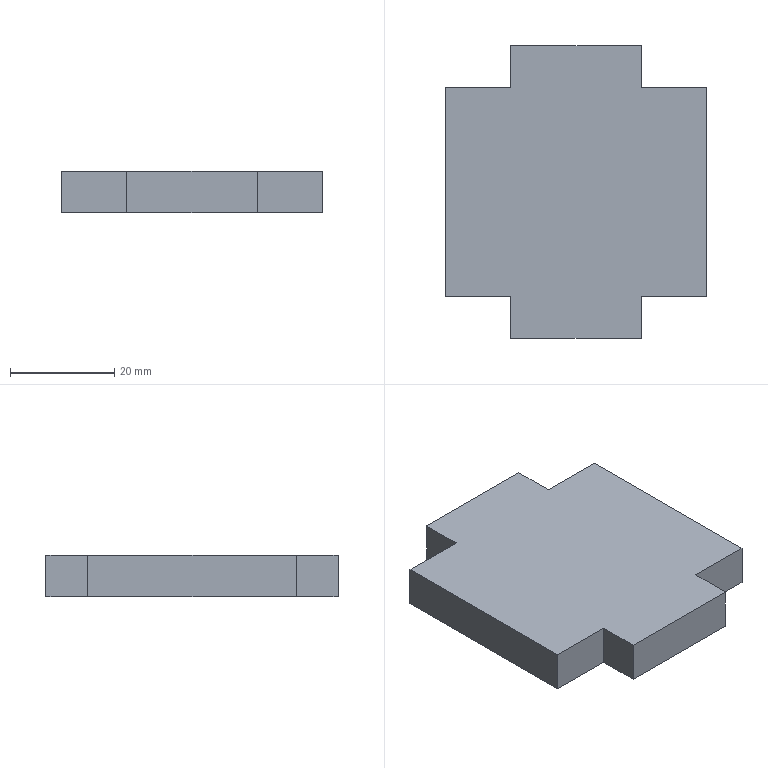Part | SolidWorks | features FlatPattern 1, SMBaseFlange 1, SheetMetal 1 | 1 solid | 14 faces | box 50 x 56 x 8 mm | volume 19200 mm3 | plane 14
STEP:
#1=CARTESIAN_POINT('',(361.372,8.,0.));
#2=VERTEX_POINT('',#1);
#3=CARTESIAN_POINT('',(373.872,8.,0.));
#4=VERTEX_POINT('',#3);
#5=CARTESIAN_POINT('',(373.872,8.,0.));
#6=DIRECTION('',(1.,0.,0.));
#7=VECTOR('',#6,1000.);
#8=LINE('',#5,#7);
#9=EDGE_CURVE('',#2,#4,#8,.T.);
#10=ORIENTED_EDGE('',*,*,#9,.F.);
#11=CARTESIAN_POINT('',(361.372,8.,-8.));
#12=VERTEX_POINT('',#11);
#13=CARTESIAN_POINT('',(361.372,8.,-8.));
#14=DIRECTION('',(0.,0.,1.));
#15=VECTOR('',#14,1000.);
#16=LINE('',#13,#15);
#17=EDGE_CURVE('',#12,#2,#16,.T.);
#18=ORIENTED_EDGE('',*,*,#17,.F.);
#19=CARTESIAN_POINT('',(373.872,8.,-8.));
#20=VERTEX_POINT('',#19);
#21=CARTESIAN_POINT('',(373.872,8.,-8.));
#22=DIRECTION('',(1.,0.,0.));
#23=VECTOR('',#22,1000.);
#24=LINE('',#21,#23);
#25=EDGE_CURVE('',#12,#20,#24,.T.);
#26=ORIENTED_EDGE('',*,*,#25,.T.);
#27=CARTESIAN_POINT('',(373.872,8.,-8.));
#28=DIRECTION('',(0.,0.,1.));
#29=VECTOR('',#28,1000.);
#30=LINE('',#27,#29);
#31=EDGE_CURVE('',#20,#4,#30,.T.);
#32=ORIENTED_EDGE('',*,*,#31,.T.);
#33=EDGE_LOOP('',(#10,#18,#26,#32));
#34=FACE_OUTER_BOUND('',#33,.T.);
#35=CARTESIAN_POINT('',(373.872,8.,-8.));
#36=DIRECTION('',(0.,-1.,0.));
#37=DIRECTION('',(1.,0.,0.));
#38=AXIS2_PLACEMENT_3D('',#35,#36,#37);
#39=PLANE('',#38);
#40=ADVANCED_FACE('',(#34),#39,.T.);
#41=CARTESIAN_POINT('',(361.372,48.,0.));
#42=VERTEX_POINT('',#41);
#43=CARTESIAN_POINT('',(361.372,8.,0.));
#44=DIRECTION('',(0.,-1.,0.));
#45=VECTOR('',#44,1000.);
#46=LINE('',#43,#45);
#47=EDGE_CURVE('',#42,#2,#46,.T.);
#48=ORIENTED_EDGE('',*,*,#47,.F.);
#49=CARTESIAN_POINT('',(361.372,48.,-8.));
#50=VERTEX_POINT('',#49);
#51=CARTESIAN_POINT('',(361.372,48.,-8.));
#52=DIRECTION('',(0.,0.,1.));
#53=VECTOR('',#52,1000.);
#54=LINE('',#51,#53);
#55=EDGE_CURVE('',#50,#42,#54,.T.);
#56=ORIENTED_EDGE('',*,*,#55,.F.);
#57=CARTESIAN_POINT('',(361.372,8.,-8.));
#58=DIRECTION('',(0.,-1.,0.));
#59=VECTOR('',#58,1000.);
#60=LINE('',#57,#59);
#61=EDGE_CURVE('',#50,#12,#60,.T.);
#62=ORIENTED_EDGE('',*,*,#61,.T.);
#63=ORIENTED_EDGE('',*,*,#17,.T.);
#64=EDGE_LOOP('',(#48,#56,#62,#63));
#65=FACE_OUTER_BOUND('',#64,.T.);
#66=CARTESIAN_POINT('',(361.372,8.,-8.));
#67=DIRECTION('',(-1.,0.,0.));
#68=DIRECTION('',(0.,-1.,0.));
#69=AXIS2_PLACEMENT_3D('',#66,#67,#68);
#70=PLANE('',#69);
#71=ADVANCED_FACE('',(#65),#70,.T.);
#72=CARTESIAN_POINT('',(373.872,48.,0.));
#73=VERTEX_POINT('',#72);
#74=CARTESIAN_POINT('',(361.372,48.,0.));
#75=DIRECTION('',(-1.,0.,0.));
#76=VECTOR('',#75,1000.);
#77=LINE('',#74,#76);
#78=EDGE_CURVE('',#73,#42,#77,.T.);
#79=ORIENTED_EDGE('',*,*,#78,.F.);
#80=CARTESIAN_POINT('',(373.872,48.,-8.));
#81=VERTEX_POINT('',#80);
#82=CARTESIAN_POINT('',(373.872,48.,-8.));
#83=DIRECTION('',(0.,0.,1.));
#84=VECTOR('',#83,1000.);
#85=LINE('',#82,#84);
#86=EDGE_CURVE('',#81,#73,#85,.T.);
#87=ORIENTED_EDGE('',*,*,#86,.F.);
#88=CARTESIAN_POINT('',(361.372,48.,-8.));
#89=DIRECTION('',(-1.,0.,0.));
#90=VECTOR('',#89,1000.);
#91=LINE('',#88,#90);
#92=EDGE_CURVE('',#81,#50,#91,.T.);
#93=ORIENTED_EDGE('',*,*,#92,.T.);
#94=ORIENTED_EDGE('',*,*,#55,.T.);
#95=EDGE_LOOP('',(#79,#87,#93,#94));
#96=FACE_OUTER_BOUND('',#95,.T.);
#97=CARTESIAN_POINT('',(361.372,48.,-8.));
#98=DIRECTION('',(0.,1.,0.));
#99=DIRECTION('',(-1.,0.,0.));
#100=AXIS2_PLACEMENT_3D('',#97,#98,#99);
#101=PLANE('',#100);
#102=ADVANCED_FACE('',(#96),#101,.T.);
#103=CARTESIAN_POINT('',(373.872,56.,0.));
#104=VERTEX_POINT('',#103);
#105=CARTESIAN_POINT('',(373.872,48.,0.));
#106=DIRECTION('',(0.,-1.,0.));
#107=VECTOR('',#106,1000.);
#108=LINE('',#105,#107);
#109=EDGE_CURVE('',#104,#73,#108,.T.);
#110=ORIENTED_EDGE('',*,*,#109,.F.);
#111=CARTESIAN_POINT('',(373.872,56.,-8.));
#112=VERTEX_POINT('',#111);
#113=CARTESIAN_POINT('',(373.872,56.,-8.));
#114=DIRECTION('',(0.,0.,1.));
#115=VECTOR('',#114,1000.);
#116=LINE('',#113,#115);
#117=EDGE_CURVE('',#112,#104,#116,.T.);
#118=ORIENTED_EDGE('',*,*,#117,.F.);
#119=CARTESIAN_POINT('',(373.872,48.,-8.));
#120=DIRECTION('',(0.,-1.,0.));
#121=VECTOR('',#120,1000.);
#122=LINE('',#119,#121);
#123=EDGE_CURVE('',#112,#81,#122,.T.);
#124=ORIENTED_EDGE('',*,*,#123,.T.);
#125=ORIENTED_EDGE('',*,*,#86,.T.);
#126=EDGE_LOOP('',(#110,#118,#124,#125));
#127=FACE_OUTER_BOUND('',#126,.T.);
#128=CARTESIAN_POINT('',(373.872,48.,-8.));
#129=DIRECTION('',(-1.,0.,0.));
#130=DIRECTION('',(0.,0.,1.));
#131=AXIS2_PLACEMENT_3D('',#128,#129,#130);
#132=PLANE('',#131);
#133=ADVANCED_FACE('',(#127),#132,.T.);
#134=CARTESIAN_POINT('',(398.872,56.,0.));
#135=VERTEX_POINT('',#134);
#136=CARTESIAN_POINT('',(373.872,56.,0.));
#137=DIRECTION('',(-1.,0.,0.));
#138=VECTOR('',#137,1000.);
#139=LINE('',#136,#138);
#140=EDGE_CURVE('',#135,#104,#139,.T.);
#141=ORIENTED_EDGE('',*,*,#140,.F.);
#142=CARTESIAN_POINT('',(398.872,56.,-8.));
#143=VERTEX_POINT('',#142);
#144=CARTESIAN_POINT('',(398.872,56.,-8.));
#145=DIRECTION('',(0.,0.,1.));
#146=VECTOR('',#145,1000.);
#147=LINE('',#144,#146);
#148=EDGE_CURVE('',#143,#135,#147,.T.);
#149=ORIENTED_EDGE('',*,*,#148,.F.);
#150=CARTESIAN_POINT('',(373.872,56.,-8.));
#151=DIRECTION('',(-1.,0.,0.));
#152=VECTOR('',#151,1000.);
#153=LINE('',#150,#152);
#154=EDGE_CURVE('',#143,#112,#153,.T.);
#155=ORIENTED_EDGE('',*,*,#154,.T.);
#156=ORIENTED_EDGE('',*,*,#117,.T.);
#157=EDGE_LOOP('',(#141,#149,#155,#156));
#158=FACE_OUTER_BOUND('',#157,.T.);
#159=CARTESIAN_POINT('',(373.872,56.,-8.));
#160=DIRECTION('',(0.,1.,0.));
#161=DIRECTION('',(0.,0.,1.));
#162=AXIS2_PLACEMENT_3D('',#159,#160,#161);
#163=PLANE('',#162);
#164=ADVANCED_FACE('',(#158),#163,.T.);
#165=CARTESIAN_POINT('',(398.872,48.,0.));
#166=VERTEX_POINT('',#165);
#167=CARTESIAN_POINT('',(398.872,56.,0.));
#168=DIRECTION('',(0.,1.,0.));
#169=VECTOR('',#168,1000.);
#170=LINE('',#167,#169);
#171=EDGE_CURVE('',#166,#135,#170,.T.);
#172=ORIENTED_EDGE('',*,*,#171,.F.);
#173=CARTESIAN_POINT('',(398.872,48.,-8.));
#174=VERTEX_POINT('',#173);
#175=CARTESIAN_POINT('',(398.872,48.,-8.));
#176=DIRECTION('',(0.,0.,1.));
#177=VECTOR('',#176,1000.);
#178=LINE('',#175,#177);
#179=EDGE_CURVE('',#174,#166,#178,.T.);
#180=ORIENTED_EDGE('',*,*,#179,.F.);
#181=CARTESIAN_POINT('',(398.872,56.,-8.));
#182=DIRECTION('',(0.,1.,0.));
#183=VECTOR('',#182,1000.);
#184=LINE('',#181,#183);
#185=EDGE_CURVE('',#174,#143,#184,.T.);
#186=ORIENTED_EDGE('',*,*,#185,.T.);
#187=ORIENTED_EDGE('',*,*,#148,.T.);
#188=EDGE_LOOP('',(#172,#180,#186,#187));
#189=FACE_OUTER_BOUND('',#188,.T.);
#190=CARTESIAN_POINT('',(398.872,56.,-8.));
#191=DIRECTION('',(1.,0.,0.));
#192=DIRECTION('',(0.,0.,-1.));
#193=AXIS2_PLACEMENT_3D('',#190,#191,#192);
#194=PLANE('',#193);
#195=ADVANCED_FACE('',(#189),#194,.T.);
#196=CARTESIAN_POINT('',(411.372,48.,0.));
#197=VERTEX_POINT('',#196);
#198=CARTESIAN_POINT('',(398.872,48.,0.));
#199=DIRECTION('',(-1.,0.,0.));
#200=VECTOR('',#199,1000.);
#201=LINE('',#198,#200);
#202=EDGE_CURVE('',#197,#166,#201,.T.);
#203=ORIENTED_EDGE('',*,*,#202,.F.);
#204=CARTESIAN_POINT('',(411.372,48.,-8.));
#205=VERTEX_POINT('',#204);
#206=CARTESIAN_POINT('',(411.372,48.,-8.));
#207=DIRECTION('',(0.,0.,1.));
#208=VECTOR('',#207,1000.);
#209=LINE('',#206,#208);
#210=EDGE_CURVE('',#205,#197,#209,.T.);
#211=ORIENTED_EDGE('',*,*,#210,.F.);
#212=CARTESIAN_POINT('',(398.872,48.,-8.));
#213=DIRECTION('',(-1.,0.,0.));
#214=VECTOR('',#213,1000.);
#215=LINE('',#212,#214);
#216=EDGE_CURVE('',#205,#174,#215,.T.);
#217=ORIENTED_EDGE('',*,*,#216,.T.);
#218=ORIENTED_EDGE('',*,*,#179,.T.);
#219=EDGE_LOOP('',(#203,#211,#217,#218));
#220=FACE_OUTER_BOUND('',#219,.T.);
#221=CARTESIAN_POINT('',(398.872,48.,-8.));
#222=DIRECTION('',(0.,1.,0.));
#223=DIRECTION('',(0.,0.,1.));
#224=AXIS2_PLACEMENT_3D('',#221,#222,#223);
#225=PLANE('',#224);
#226=ADVANCED_FACE('',(#220),#225,.T.);
#227=CARTESIAN_POINT('',(411.372,8.,0.));
#228=VERTEX_POINT('',#227);
#229=CARTESIAN_POINT('',(411.372,48.,0.));
#230=DIRECTION('',(0.,1.,0.));
#231=VECTOR('',#230,1000.);
#232=LINE('',#229,#231);
#233=EDGE_CURVE('',#228,#197,#232,.T.);
#234=ORIENTED_EDGE('',*,*,#233,.F.);
#235=CARTESIAN_POINT('',(411.372,8.,-8.));
#236=VERTEX_POINT('',#235);
#237=CARTESIAN_POINT('',(411.372,8.,-8.));
#238=DIRECTION('',(0.,0.,1.));
#239=VECTOR('',#238,1000.);
#240=LINE('',#237,#239);
#241=EDGE_CURVE('',#236,#228,#240,.T.);
#242=ORIENTED_EDGE('',*,*,#241,.F.);
#243=CARTESIAN_POINT('',(411.372,48.,-8.));
#244=DIRECTION('',(0.,1.,0.));
#245=VECTOR('',#244,1000.);
#246=LINE('',#243,#245);
#247=EDGE_CURVE('',#236,#205,#246,.T.);
#248=ORIENTED_EDGE('',*,*,#247,.T.);
#249=ORIENTED_EDGE('',*,*,#210,.T.);
#250=EDGE_LOOP('',(#234,#242,#248,#249));
#251=FACE_OUTER_BOUND('',#250,.T.);
#252=CARTESIAN_POINT('',(411.372,48.,-8.));
#253=DIRECTION('',(1.,0.,0.));
#254=DIRECTION('',(0.,1.,0.));
#255=AXIS2_PLACEMENT_3D('',#252,#253,#254);
#256=PLANE('',#255);
#257=ADVANCED_FACE('',(#251),#256,.T.);
#258=CARTESIAN_POINT('',(398.872,8.,0.));
#259=VERTEX_POINT('',#258);
#260=CARTESIAN_POINT('',(411.372,8.,0.));
#261=DIRECTION('',(1.,0.,0.));
#262=VECTOR('',#261,1000.);
#263=LINE('',#260,#262);
#264=EDGE_CURVE('',#259,#228,#263,.T.);
#265=ORIENTED_EDGE('',*,*,#264,.F.);
#266=CARTESIAN_POINT('',(398.872,8.,-8.));
#267=VERTEX_POINT('',#266);
#268=CARTESIAN_POINT('',(398.872,8.,-8.));
#269=DIRECTION('',(0.,0.,1.));
#270=VECTOR('',#269,1000.);
#271=LINE('',#268,#270);
#272=EDGE_CURVE('',#267,#259,#271,.T.);
#273=ORIENTED_EDGE('',*,*,#272,.F.);
#274=CARTESIAN_POINT('',(411.372,8.,-8.));
#275=DIRECTION('',(1.,0.,0.));
#276=VECTOR('',#275,1000.);
#277=LINE('',#274,#276);
#278=EDGE_CURVE('',#267,#236,#277,.T.);
#279=ORIENTED_EDGE('',*,*,#278,.T.);
#280=ORIENTED_EDGE('',*,*,#241,.T.);
#281=EDGE_LOOP('',(#265,#273,#279,#280));
#282=FACE_OUTER_BOUND('',#281,.T.);
#283=CARTESIAN_POINT('',(411.372,8.,-8.));
#284=DIRECTION('',(0.,-1.,0.));
#285=DIRECTION('',(1.,0.,0.));
#286=AXIS2_PLACEMENT_3D('',#283,#284,#285);
#287=PLANE('',#286);
#288=ADVANCED_FACE('',(#282),#287,.T.);
#289=CARTESIAN_POINT('',(398.872,0.,0.));
#290=VERTEX_POINT('',#289);
#291=CARTESIAN_POINT('',(398.872,8.,0.));
#292=DIRECTION('',(0.,1.,0.));
#293=VECTOR('',#292,1000.);
#294=LINE('',#291,#293);
#295=EDGE_CURVE('',#290,#259,#294,.T.);
#296=ORIENTED_EDGE('',*,*,#295,.F.);
#297=CARTESIAN_POINT('',(398.872,0.,-8.));
#298=VERTEX_POINT('',#297);
#299=CARTESIAN_POINT('',(398.872,0.,-8.));
#300=DIRECTION('',(0.,0.,1.));
#301=VECTOR('',#300,1000.);
#302=LINE('',#299,#301);
#303=EDGE_CURVE('',#298,#290,#302,.T.);
#304=ORIENTED_EDGE('',*,*,#303,.F.);
#305=CARTESIAN_POINT('',(398.872,8.,-8.));
#306=DIRECTION('',(0.,1.,0.));
#307=VECTOR('',#306,1000.);
#308=LINE('',#305,#307);
#309=EDGE_CURVE('',#298,#267,#308,.T.);
#310=ORIENTED_EDGE('',*,*,#309,.T.);
#311=ORIENTED_EDGE('',*,*,#272,.T.);
#312=EDGE_LOOP('',(#296,#304,#310,#311));
#313=FACE_OUTER_BOUND('',#312,.T.);
#314=CARTESIAN_POINT('',(398.872,8.,-8.));
#315=DIRECTION('',(1.,0.,0.));
#316=DIRECTION('',(0.,0.,-1.));
#317=AXIS2_PLACEMENT_3D('',#314,#315,#316);
#318=PLANE('',#317);
#319=ADVANCED_FACE('',(#313),#318,.T.);
#320=CARTESIAN_POINT('',(373.872,0.,0.));
#321=VERTEX_POINT('',#320);
#322=CARTESIAN_POINT('',(398.872,0.,0.));
#323=DIRECTION('',(1.,0.,0.));
#324=VECTOR('',#323,1000.);
#325=LINE('',#322,#324);
#326=EDGE_CURVE('',#321,#290,#325,.T.);
#327=ORIENTED_EDGE('',*,*,#326,.F.);
#328=CARTESIAN_POINT('',(373.872,0.,-8.));
#329=VERTEX_POINT('',#328);
#330=CARTESIAN_POINT('',(373.872,0.,-8.));
#331=DIRECTION('',(0.,0.,1.));
#332=VECTOR('',#331,1000.);
#333=LINE('',#330,#332);
#334=EDGE_CURVE('',#329,#321,#333,.T.);
#335=ORIENTED_EDGE('',*,*,#334,.F.);
#336=CARTESIAN_POINT('',(398.872,0.,-8.));
#337=DIRECTION('',(1.,0.,0.));
#338=VECTOR('',#337,1000.);
#339=LINE('',#336,#338);
#340=EDGE_CURVE('',#329,#298,#339,.T.);
#341=ORIENTED_EDGE('',*,*,#340,.T.);
#342=ORIENTED_EDGE('',*,*,#303,.T.);
#343=EDGE_LOOP('',(#327,#335,#341,#342));
#344=FACE_OUTER_BOUND('',#343,.T.);
#345=CARTESIAN_POINT('',(398.872,0.,-8.));
#346=DIRECTION('',(0.,-1.,0.));
#347=DIRECTION('',(0.,0.,-1.));
#348=AXIS2_PLACEMENT_3D('',#345,#346,#347);
#349=PLANE('',#348);
#350=ADVANCED_FACE('',(#344),#349,.T.);
#351=CARTESIAN_POINT('',(373.872,0.,0.));
#352=DIRECTION('',(0.,-1.,0.));
#353=VECTOR('',#352,1000.);
#354=LINE('',#351,#353);
#355=EDGE_CURVE('',#4,#321,#354,.T.);
#356=ORIENTED_EDGE('',*,*,#355,.F.);
#357=ORIENTED_EDGE('',*,*,#31,.F.);
#358=CARTESIAN_POINT('',(373.872,0.,-8.));
#359=DIRECTION('',(0.,-1.,0.));
#360=VECTOR('',#359,1000.);
#361=LINE('',#358,#360);
#362=EDGE_CURVE('',#20,#329,#361,.T.);
#363=ORIENTED_EDGE('',*,*,#362,.T.);
#364=ORIENTED_EDGE('',*,*,#334,.T.);
#365=EDGE_LOOP('',(#356,#357,#363,#364));
#366=FACE_OUTER_BOUND('',#365,.T.);
#367=CARTESIAN_POINT('',(373.872,0.,-8.));
#368=DIRECTION('',(-1.,0.,0.));
#369=DIRECTION('',(0.,0.,1.));
#370=AXIS2_PLACEMENT_3D('',#367,#368,#369);
#371=PLANE('',#370);
#372=ADVANCED_FACE('',(#366),#371,.T.);
#373=ORIENTED_EDGE('',*,*,#25,.F.);
#374=ORIENTED_EDGE('',*,*,#61,.F.);
#375=ORIENTED_EDGE('',*,*,#92,.F.);
#376=ORIENTED_EDGE('',*,*,#123,.F.);
#377=ORIENTED_EDGE('',*,*,#154,.F.);
#378=ORIENTED_EDGE('',*,*,#185,.F.);
#379=ORIENTED_EDGE('',*,*,#216,.F.);
#380=ORIENTED_EDGE('',*,*,#247,.F.);
#381=ORIENTED_EDGE('',*,*,#278,.F.);
#382=ORIENTED_EDGE('',*,*,#309,.F.);
#383=ORIENTED_EDGE('',*,*,#340,.F.);
#384=ORIENTED_EDGE('',*,*,#362,.F.);
#385=EDGE_LOOP('',(#373,#374,#375,#376,#377,#378,#379,#380,#381,#382,#383,#384));
#386=FACE_OUTER_BOUND('',#385,.T.);
#387=CARTESIAN_POINT('',(0.,0.,-8.));
#388=DIRECTION('',(0.,0.,-1.));
#389=DIRECTION('',(-1.,0.,0.));
#390=AXIS2_PLACEMENT_3D('',#387,#388,#389);
#391=PLANE('',#390);
#392=ADVANCED_FACE('',(#386),#391,.T.);
#393=ORIENTED_EDGE('',*,*,#9,.T.);
#394=ORIENTED_EDGE('',*,*,#355,.T.);
#395=ORIENTED_EDGE('',*,*,#326,.T.);
#396=ORIENTED_EDGE('',*,*,#295,.T.);
#397=ORIENTED_EDGE('',*,*,#264,.T.);
#398=ORIENTED_EDGE('',*,*,#233,.T.);
#399=ORIENTED_EDGE('',*,*,#202,.T.);
#400=ORIENTED_EDGE('',*,*,#171,.T.);
#401=ORIENTED_EDGE('',*,*,#140,.T.);
#402=ORIENTED_EDGE('',*,*,#109,.T.);
#403=ORIENTED_EDGE('',*,*,#78,.T.);
#404=ORIENTED_EDGE('',*,*,#47,.T.);
#405=EDGE_LOOP('',(#393,#394,#395,#396,#397,#398,#399,#400,#401,#402,#403,#404));
#406=FACE_OUTER_BOUND('',#405,.T.);
#407=CARTESIAN_POINT('',(0.,0.,0.));
#408=DIRECTION('',(0.,0.,-1.));
#409=DIRECTION('',(-1.,0.,0.));
#410=AXIS2_PLACEMENT_3D('',#407,#408,#409);
#411=PLANE('',#410);
#412=ADVANCED_FACE('',(#406),#411,.F.);
#413=CLOSED_SHELL('',(#40,#71,#102,#133,#164,#195,#226,#257,#288,#319,#350,#372,#392,#412));
#414=MANIFOLD_SOLID_BREP('',#413);
#415=CARTESIAN_POINT('',(0.,0.,0.));
#416=DIRECTION('',(0.,0.,1.));
#417=DIRECTION('',(1.,0.,0.));
#418=AXIS2_PLACEMENT_3D('',#415,#416,#417);
#419=(LENGTH_UNIT()NAMED_UNIT(*)SI_UNIT(.MILLI.,.METRE.));
#420=UNCERTAINTY_MEASURE_WITH_UNIT(LENGTH_MEASURE(0.00001),#419,'','');
#421=(NAMED_UNIT(*)PLANE_ANGLE_UNIT()SI_UNIT($,.RADIAN.));
#422=(NAMED_UNIT(*)SI_UNIT($,.STERADIAN.)SOLID_ANGLE_UNIT());
#423=(GEOMETRIC_REPRESENTATION_CONTEXT(3)GLOBAL_UNCERTAINTY_ASSIGNED_CONTEXT((#420))GLOBAL_UNIT_ASSIGNED_CONTEXT((#419,#421,#422))REPRESENTATION_CONTEXT('',''));
#424=ADVANCED_BREP_SHAPE_REPRESENTATION('',(#414,#418),#423);